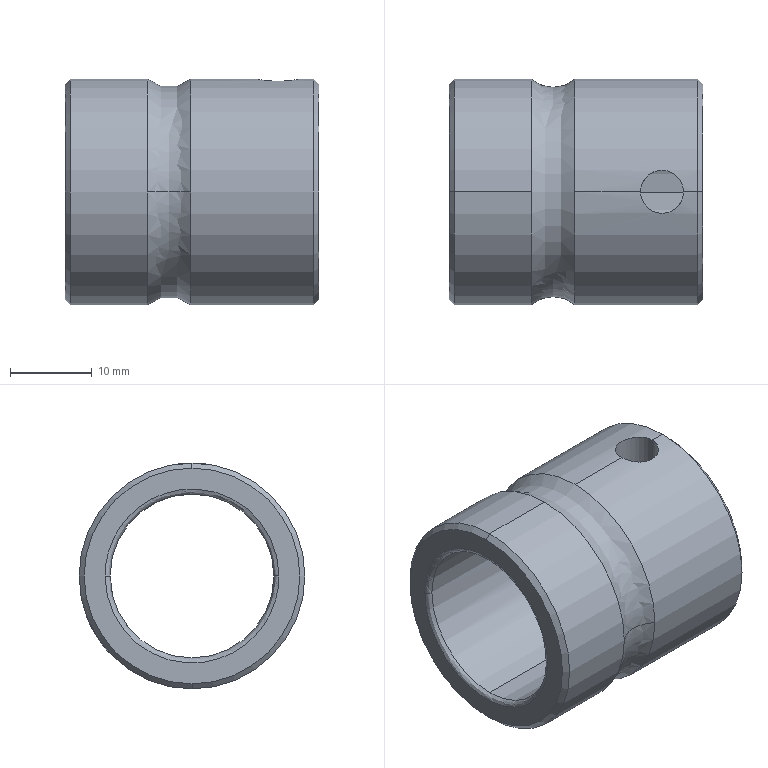Part | STEP file | Microwave Drying Flat Conveyor-inafag_ucfl204_62o9y6gnj3059x015y4y3bh4_03 | 1 solid | 22 faces | box 31 x 27.56 x 27.56 mm | volume 8243 mm3 | cylinder 10 | spline 6 | cone 4 | plane 2 | commonest cylinder face diameters 5.25 x4 27.56 x4 20 x2
STEP:
#1=CARTESIAN_POINT('',(2.3,10.62,0.));
#2=VERTEX_POINT('',#1);
#3=CARTESIAN_POINT('',(2.3,-10.62,0.));
#4=VERTEX_POINT('',#3);
#5=CARTESIAN_POINT('',(2.3,10.62,0.));
#6=CARTESIAN_POINT('',(2.3,10.62,-21.24));
#7=CARTESIAN_POINT('',(2.3,-10.62,-21.24));
#8=CARTESIAN_POINT('',(2.3,-10.62,0.));
#9=(BOUNDED_CURVE()B_SPLINE_CURVE(3,(#5,#6,#7,#8),.UNSPECIFIED.,.F.,.F.)B_SPLINE_CURVE_WITH_KNOTS((4,4),(0.25,0.75),.UNSPECIFIED.)CURVE()GEOMETRIC_REPRESENTATION_ITEM()RATIONAL_B_SPLINE_CURVE((1.,0.3333,0.3333,1.))REPRESENTATION_ITEM(''));
#10=EDGE_CURVE('',#2,#4,#9,.T.);
#11=ORIENTED_EDGE('',*,*,#10,.T.);
#12=CARTESIAN_POINT('',(2.92,-10.,0.));
#13=VERTEX_POINT('',#12);
#14=CARTESIAN_POINT('',(2.92,-10.62,0.));
#15=DIRECTION('',(0.,0.,-1.));
#16=DIRECTION('',(0.,-1.,0.));
#17=AXIS2_PLACEMENT_3D('',#14,#15,#16);
#18=CIRCLE('',#17,0.62);
#19=EDGE_CURVE('',#4,#13,#18,.T.);
#20=ORIENTED_EDGE('',*,*,#19,.T.);
#21=CARTESIAN_POINT('',(2.92,0.,-10.));
#22=VERTEX_POINT('',#21);
#23=CARTESIAN_POINT('',(2.92,0.,0.));
#24=DIRECTION('',(-1.,0.,0.));
#25=DIRECTION('',(0.,0.,1.));
#26=AXIS2_PLACEMENT_3D('',#23,#24,#25);
#27=CIRCLE('',#26,10.);
#28=EDGE_CURVE('',#22,#13,#27,.T.);
#29=ORIENTED_EDGE('',*,*,#28,.F.);
#30=CARTESIAN_POINT('',(2.92,10.,0.));
#31=VERTEX_POINT('',#30);
#32=CARTESIAN_POINT('',(2.92,0.,0.));
#33=DIRECTION('',(-1.,0.,0.));
#34=DIRECTION('',(0.,0.,1.));
#35=AXIS2_PLACEMENT_3D('',#32,#33,#34);
#36=CIRCLE('',#35,10.);
#37=EDGE_CURVE('',#31,#22,#36,.T.);
#38=ORIENTED_EDGE('',*,*,#37,.F.);
#39=CARTESIAN_POINT('',(2.92,10.62,0.));
#40=DIRECTION('',(0.,0.,1.));
#41=DIRECTION('',(0.,1.,0.));
#42=AXIS2_PLACEMENT_3D('',#39,#40,#41);
#43=CIRCLE('',#42,0.62);
#44=EDGE_CURVE('',#2,#31,#43,.T.);
#45=ORIENTED_EDGE('',*,*,#44,.F.);
#46=EDGE_LOOP('',(#11,#20,#29,#38,#45));
#47=FACE_OUTER_BOUND('',#46,.T.);
#48=CARTESIAN_POINT('',(2.3,-10.62,0.));
#49=CARTESIAN_POINT('',(2.3,-10.62,-21.24));
#50=CARTESIAN_POINT('',(2.3,10.62,-21.24));
#51=CARTESIAN_POINT('',(2.3,10.62,0.));
#52=CARTESIAN_POINT('',(2.3,-10.257,0.));
#53=CARTESIAN_POINT('',(2.3,-10.257,-20.514));
#54=CARTESIAN_POINT('',(2.3,10.257,-20.514));
#55=CARTESIAN_POINT('',(2.3,10.257,0.));
#56=CARTESIAN_POINT('',(2.557,-10.,0.));
#57=CARTESIAN_POINT('',(2.557,-10.,-20.));
#58=CARTESIAN_POINT('',(2.557,10.,-20.));
#59=CARTESIAN_POINT('',(2.557,10.,0.));
#60=CARTESIAN_POINT('',(2.92,-10.,0.));
#61=CARTESIAN_POINT('',(2.92,-10.,-20.));
#62=CARTESIAN_POINT('',(2.92,10.,-20.));
#63=CARTESIAN_POINT('',(2.92,10.,0.));
#64=(BOUNDED_SURFACE()B_SPLINE_SURFACE(3,3,((#48,#49,#50,#51),(#52,#53,#54,#55),(#56,#57,#58,#59),(#60,#61,#62,#63)),.UNSPECIFIED.,.F.,.F.,.T.)B_SPLINE_SURFACE_WITH_KNOTS((4,4),(4,4),(0.,1.),(0.,1.),.UNSPECIFIED.)GEOMETRIC_REPRESENTATION_ITEM()RATIONAL_B_SPLINE_SURFACE(((1.,0.3333,0.3333,1.),(0.8047,0.2682,0.2682,0.8047),(0.8047,0.2682,0.2682,0.8047),(1.,0.3333,0.3333,1.)))REPRESENTATION_ITEM('')SURFACE());
#65=ADVANCED_FACE('',(#47),#64,.T.);
#66=CARTESIAN_POINT('',(32.68,-10.,0.));
#67=VERTEX_POINT('',#66);
#68=CARTESIAN_POINT('',(32.68,0.,-10.));
#69=VERTEX_POINT('',#68);
#70=CARTESIAN_POINT('',(32.68,0.,0.));
#71=DIRECTION('',(1.,0.,0.));
#72=DIRECTION('',(0.,0.,1.));
#73=AXIS2_PLACEMENT_3D('',#70,#71,#72);
#74=CIRCLE('',#73,10.);
#75=EDGE_CURVE('',#67,#69,#74,.T.);
#76=ORIENTED_EDGE('',*,*,#75,.F.);
#77=CARTESIAN_POINT('',(33.3,-10.62,0.));
#78=VERTEX_POINT('',#77);
#79=CARTESIAN_POINT('',(32.68,-10.62,0.));
#80=DIRECTION('',(0.,0.,-1.));
#81=DIRECTION('',(0.,-1.,0.));
#82=AXIS2_PLACEMENT_3D('',#79,#80,#81);
#83=CIRCLE('',#82,0.62);
#84=EDGE_CURVE('',#67,#78,#83,.T.);
#85=ORIENTED_EDGE('',*,*,#84,.T.);
#86=CARTESIAN_POINT('',(33.3,10.62,0.));
#87=VERTEX_POINT('',#86);
#88=CARTESIAN_POINT('',(33.3,-10.62,0.));
#89=CARTESIAN_POINT('',(33.3,-10.62,-21.24));
#90=CARTESIAN_POINT('',(33.3,10.62,-21.24));
#91=CARTESIAN_POINT('',(33.3,10.62,0.));
#92=(BOUNDED_CURVE()B_SPLINE_CURVE(3,(#88,#89,#90,#91),.UNSPECIFIED.,.F.,.F.)B_SPLINE_CURVE_WITH_KNOTS((4,4),(0.25,0.75),.UNSPECIFIED.)CURVE()GEOMETRIC_REPRESENTATION_ITEM()RATIONAL_B_SPLINE_CURVE((1.,0.3333,0.3333,1.))REPRESENTATION_ITEM(''));
#93=EDGE_CURVE('',#78,#87,#92,.T.);
#94=ORIENTED_EDGE('',*,*,#93,.T.);
#95=CARTESIAN_POINT('',(32.68,10.,0.));
#96=VERTEX_POINT('',#95);
#97=CARTESIAN_POINT('',(32.68,10.62,0.));
#98=DIRECTION('',(0.,0.,1.));
#99=DIRECTION('',(0.,1.,0.));
#100=AXIS2_PLACEMENT_3D('',#97,#98,#99);
#101=CIRCLE('',#100,0.62);
#102=EDGE_CURVE('',#96,#87,#101,.T.);
#103=ORIENTED_EDGE('',*,*,#102,.F.);
#104=CARTESIAN_POINT('',(32.68,0.,0.));
#105=DIRECTION('',(1.,0.,0.));
#106=DIRECTION('',(0.,0.,1.));
#107=AXIS2_PLACEMENT_3D('',#104,#105,#106);
#108=CIRCLE('',#107,10.);
#109=EDGE_CURVE('',#69,#96,#108,.T.);
#110=ORIENTED_EDGE('',*,*,#109,.F.);
#111=EDGE_LOOP('',(#76,#85,#94,#103,#110));
#112=FACE_OUTER_BOUND('',#111,.T.);
#113=CARTESIAN_POINT('',(32.68,-10.,0.));
#114=CARTESIAN_POINT('',(32.68,-10.,-20.));
#115=CARTESIAN_POINT('',(32.68,10.,-20.));
#116=CARTESIAN_POINT('',(32.68,10.,0.));
#117=CARTESIAN_POINT('',(33.043,-10.,0.));
#118=CARTESIAN_POINT('',(33.043,-10.,-20.));
#119=CARTESIAN_POINT('',(33.043,10.,-20.));
#120=CARTESIAN_POINT('',(33.043,10.,0.));
#121=CARTESIAN_POINT('',(33.3,-10.257,0.));
#122=CARTESIAN_POINT('',(33.3,-10.257,-20.514));
#123=CARTESIAN_POINT('',(33.3,10.257,-20.514));
#124=CARTESIAN_POINT('',(33.3,10.257,0.));
#125=CARTESIAN_POINT('',(33.3,-10.62,0.));
#126=CARTESIAN_POINT('',(33.3,-10.62,-21.24));
#127=CARTESIAN_POINT('',(33.3,10.62,-21.24));
#128=CARTESIAN_POINT('',(33.3,10.62,0.));
#129=(BOUNDED_SURFACE()B_SPLINE_SURFACE(3,3,((#113,#114,#115,#116),(#117,#118,#119,#120),(#121,#122,#123,#124),(#125,#126,#127,#128)),.UNSPECIFIED.,.F.,.F.,.F.)B_SPLINE_SURFACE_WITH_KNOTS((4,4),(4,4),(0.,1.),(0.,1.),.UNSPECIFIED.)GEOMETRIC_REPRESENTATION_ITEM()RATIONAL_B_SPLINE_SURFACE(((1.,0.3333,0.3333,1.),(0.8047,0.2682,0.2682,0.8047),(0.8047,0.2682,0.2682,0.8047),(1.,0.3333,0.3333,1.)))REPRESENTATION_ITEM('')SURFACE());
#130=ADVANCED_FACE('',(#112),#129,.T.);
#131=CARTESIAN_POINT('',(17.634,-13.78,0.));
#132=VERTEX_POINT('',#131);
#133=CARTESIAN_POINT('',(17.634,0.,-13.78));
#134=VERTEX_POINT('',#133);
#135=CARTESIAN_POINT('',(17.634,0.,0.));
#136=DIRECTION('',(1.,0.,0.));
#137=DIRECTION('',(0.,0.,-1.));
#138=AXIS2_PLACEMENT_3D('',#135,#136,#137);
#139=CIRCLE('',#138,13.78);
#140=EDGE_CURVE('',#132,#134,#139,.T.);
#141=ORIENTED_EDGE('',*,*,#140,.F.);
#142=CARTESIAN_POINT('',(12.366,-13.78,0.));
#143=VERTEX_POINT('',#142);
#144=CARTESIAN_POINT('',(15.,-16.75,0.));
#145=DIRECTION('',(0.,0.,1.));
#146=DIRECTION('',(0.,-1.,0.));
#147=AXIS2_PLACEMENT_3D('',#144,#145,#146);
#148=CIRCLE('',#147,3.97);
#149=EDGE_CURVE('',#132,#143,#148,.T.);
#150=ORIENTED_EDGE('',*,*,#149,.T.);
#151=CARTESIAN_POINT('',(12.366,0.,-13.78));
#152=VERTEX_POINT('',#151);
#153=CARTESIAN_POINT('',(12.366,0.,0.));
#154=DIRECTION('',(1.,0.,0.));
#155=DIRECTION('',(0.,1.,0.));
#156=AXIS2_PLACEMENT_3D('',#153,#154,#155);
#157=CIRCLE('',#156,13.78);
#158=EDGE_CURVE('',#143,#152,#157,.T.);
#159=ORIENTED_EDGE('',*,*,#158,.T.);
#160=CARTESIAN_POINT('',(12.366,13.78,0.));
#161=VERTEX_POINT('',#160);
#162=CARTESIAN_POINT('',(12.366,0.,0.));
#163=DIRECTION('',(1.,0.,0.));
#164=DIRECTION('',(0.,1.,0.));
#165=AXIS2_PLACEMENT_3D('',#162,#163,#164);
#166=CIRCLE('',#165,13.78);
#167=EDGE_CURVE('',#152,#161,#166,.T.);
#168=ORIENTED_EDGE('',*,*,#167,.T.);
#169=CARTESIAN_POINT('',(17.634,13.78,0.));
#170=VERTEX_POINT('',#169);
#171=CARTESIAN_POINT('',(15.,16.75,0.));
#172=DIRECTION('',(0.,0.,-1.));
#173=DIRECTION('',(0.,1.,0.));
#174=AXIS2_PLACEMENT_3D('',#171,#172,#173);
#175=CIRCLE('',#174,3.97);
#176=EDGE_CURVE('',#170,#161,#175,.T.);
#177=ORIENTED_EDGE('',*,*,#176,.F.);
#178=CARTESIAN_POINT('',(17.634,0.,0.));
#179=DIRECTION('',(1.,0.,0.));
#180=DIRECTION('',(0.,0.,-1.));
#181=AXIS2_PLACEMENT_3D('',#178,#179,#180);
#182=CIRCLE('',#181,13.78);
#183=EDGE_CURVE('',#134,#170,#182,.T.);
#184=ORIENTED_EDGE('',*,*,#183,.F.);
#185=EDGE_LOOP('',(#141,#150,#159,#168,#177,#184));
#186=FACE_OUTER_BOUND('',#185,.T.);
#187=CARTESIAN_POINT('',(17.634,-13.78,0.));
#188=CARTESIAN_POINT('',(17.634,-13.78,-27.56));
#189=CARTESIAN_POINT('',(17.634,13.78,-27.56));
#190=CARTESIAN_POINT('',(17.634,13.78,0.));
#191=CARTESIAN_POINT('',(16.055,-12.379,0.));
#192=CARTESIAN_POINT('',(16.055,-12.379,-24.759));
#193=CARTESIAN_POINT('',(16.055,12.379,-24.759));
#194=CARTESIAN_POINT('',(16.055,12.379,0.));
#195=CARTESIAN_POINT('',(13.945,-12.379,0.));
#196=CARTESIAN_POINT('',(13.945,-12.379,-24.759));
#197=CARTESIAN_POINT('',(13.945,12.379,-24.759));
#198=CARTESIAN_POINT('',(13.945,12.379,0.));
#199=CARTESIAN_POINT('',(12.366,-13.78,0.));
#200=CARTESIAN_POINT('',(12.366,-13.78,-27.56));
#201=CARTESIAN_POINT('',(12.366,13.78,-27.56));
#202=CARTESIAN_POINT('',(12.366,13.78,0.));
#203=(BOUNDED_SURFACE()B_SPLINE_SURFACE(3,3,((#187,#188,#189,#190),(#191,#192,#193,#194),(#195,#196,#197,#198),(#199,#200,#201,#202)),.UNSPECIFIED.,.F.,.F.,.F.)B_SPLINE_SURFACE_WITH_KNOTS((4,4),(4,4),(0.,1.),(0.,1.),.UNSPECIFIED.)GEOMETRIC_REPRESENTATION_ITEM()RATIONAL_B_SPLINE_SURFACE(((1.,0.3333,0.3333,1.),(0.8321,0.2774,0.2774,0.8321),(0.8321,0.2774,0.2774,0.8321),(1.,0.3333,0.3333,1.)))REPRESENTATION_ITEM('')SURFACE());
#204=ADVANCED_FACE('',(#186),#203,.T.);
#205=ORIENTED_EDGE('',*,*,#28,.T.);
#206=CARTESIAN_POINT('',(2.92,0.,10.));
#207=VERTEX_POINT('',#206);
#208=CARTESIAN_POINT('',(2.92,0.,0.));
#209=DIRECTION('',(-1.,0.,0.));
#210=DIRECTION('',(0.,0.,1.));
#211=AXIS2_PLACEMENT_3D('',#208,#209,#210);
#212=CIRCLE('',#211,10.);
#213=EDGE_CURVE('',#13,#207,#212,.T.);
#214=ORIENTED_EDGE('',*,*,#213,.T.);
#215=CARTESIAN_POINT('',(25.675,0.,10.));
#216=VERTEX_POINT('',#215);
#217=CARTESIAN_POINT('',(2.92,0.,10.));
#218=DIRECTION('',(1.,0.,0.));
#219=VECTOR('',#218,1000.);
#220=LINE('',#217,#219);
#221=EDGE_CURVE('',#207,#216,#220,.T.);
#222=ORIENTED_EDGE('',*,*,#221,.T.);
#223=CARTESIAN_POINT('',(30.925,0.,10.));
#224=VERTEX_POINT('',#223);
#225=CARTESIAN_POINT('',(25.675,0.,10.));
#226=CARTESIAN_POINT('',(25.675,-0.1741,10.));
#227=CARTESIAN_POINT('',(25.692,-0.3452,9.995));
#228=CARTESIAN_POINT('',(25.759,-0.6816,9.978));
#229=CARTESIAN_POINT('',(25.81,-0.8487,9.965));
#230=CARTESIAN_POINT('',(25.942,-1.166,9.933));
#231=CARTESIAN_POINT('',(26.023,-1.317,9.914));
#232=CARTESIAN_POINT('',(26.213,-1.601,9.872));
#233=CARTESIAN_POINT('',(26.323,-1.735,9.849));
#234=CARTESIAN_POINT('',(26.684,-2.097,9.781));
#235=CARTESIAN_POINT('',(26.976,-2.292,9.735));
#236=CARTESIAN_POINT('',(27.448,-2.489,9.686));
#237=CARTESIAN_POINT('',(27.614,-2.54,9.672));
#238=CARTESIAN_POINT('',(27.954,-2.608,9.654));
#239=CARTESIAN_POINT('',(28.126,-2.625,9.649));
#240=CARTESIAN_POINT('',(28.474,-2.625,9.649));
#241=CARTESIAN_POINT('',(28.645,-2.608,9.654));
#242=CARTESIAN_POINT('',(28.982,-2.541,9.672));
#243=CARTESIAN_POINT('',(29.149,-2.49,9.685));
#244=CARTESIAN_POINT('',(29.466,-2.358,9.718));
#245=CARTESIAN_POINT('',(29.616,-2.278,9.738));
#246=CARTESIAN_POINT('',(29.901,-2.087,9.78));
#247=CARTESIAN_POINT('',(30.035,-1.977,9.803));
#248=CARTESIAN_POINT('',(30.397,-1.616,9.872));
#249=CARTESIAN_POINT('',(30.592,-1.325,9.917));
#250=CARTESIAN_POINT('',(30.789,-0.8516,9.965));
#251=CARTESIAN_POINT('',(30.84,-0.6858,9.978));
#252=CARTESIAN_POINT('',(30.908,-0.3461,9.995));
#253=CARTESIAN_POINT('',(30.925,-0.1741,10.));
#254=CARTESIAN_POINT('',(30.925,0.,10.));
#255=B_SPLINE_CURVE_WITH_KNOTS('',3,(#225,#226,#227,#228,#229,#230,#231,#232,#233,#234,#235,#236,#237,#238,#239,#240,#241,#242,#243,#244,#245,#246,#247,#248,#249,#250,#251,#252,#253,#254),.UNSPECIFIED.,.F.,.F.,(4,2,2,2,2,2,2,2,2,2,2,2,2,2,4),(0.,0.0005149,0.00103,0.001545,0.002059,0.003089,0.003604,0.004119,0.004634,0.005149,0.005663,0.006178,0.007208,0.007723,0.008238),.UNSPECIFIED.);
#256=EDGE_CURVE('',#216,#224,#255,.T.);
#257=ORIENTED_EDGE('',*,*,#256,.T.);
#258=CARTESIAN_POINT('',(32.68,0.,10.));
#259=VERTEX_POINT('',#258);
#260=CARTESIAN_POINT('',(2.92,0.,10.));
#261=DIRECTION('',(1.,0.,0.));
#262=VECTOR('',#261,1000.);
#263=LINE('',#260,#262);
#264=EDGE_CURVE('',#224,#259,#263,.T.);
#265=ORIENTED_EDGE('',*,*,#264,.T.);
#266=CARTESIAN_POINT('',(32.68,0.,0.));
#267=DIRECTION('',(1.,0.,0.));
#268=DIRECTION('',(0.,0.,1.));
#269=AXIS2_PLACEMENT_3D('',#266,#267,#268);
#270=CIRCLE('',#269,10.);
#271=EDGE_CURVE('',#259,#67,#270,.T.);
#272=ORIENTED_EDGE('',*,*,#271,.T.);
#273=ORIENTED_EDGE('',*,*,#75,.T.);
#274=CARTESIAN_POINT('',(2.92,0.,-10.));
#275=DIRECTION('',(1.,0.,0.));
#276=VECTOR('',#275,1000.);
#277=LINE('',#274,#276);
#278=EDGE_CURVE('',#22,#69,#277,.T.);
#279=ORIENTED_EDGE('',*,*,#278,.F.);
#280=EDGE_LOOP('',(#205,#214,#222,#257,#265,#272,#273,#279));
#281=FACE_OUTER_BOUND('',#280,.T.);
#282=CARTESIAN_POINT('',(2.92,0.,0.));
#283=DIRECTION('',(1.,0.,0.));
#284=DIRECTION('',(0.,0.,-1.));
#285=AXIS2_PLACEMENT_3D('',#282,#283,#284);
#286=CYLINDRICAL_SURFACE('',#285,10.);
#287=ADVANCED_FACE('',(#281),#286,.F.);
#288=ORIENTED_EDGE('',*,*,#256,.F.);
#289=CARTESIAN_POINT('',(25.675,0.,13.78));
#290=VERTEX_POINT('',#289);
#291=CARTESIAN_POINT('',(25.675,0.,13.78));
#292=DIRECTION('',(0.,0.,1.));
#293=VECTOR('',#292,1000.);
#294=LINE('',#291,#293);
#295=EDGE_CURVE('',#216,#290,#294,.T.);
#296=ORIENTED_EDGE('',*,*,#295,.T.);
#297=CARTESIAN_POINT('',(30.925,0.,13.78));
#298=VERTEX_POINT('',#297);
#299=CARTESIAN_POINT('',(30.925,0.,13.78));
#300=CARTESIAN_POINT('',(30.925,-0.1737,13.78));
#301=CARTESIAN_POINT('',(30.908,-0.3445,13.777));
#302=CARTESIAN_POINT('',(30.841,-0.6804,13.764));
#303=CARTESIAN_POINT('',(30.79,-0.8472,13.755));
#304=CARTESIAN_POINT('',(30.659,-1.165,13.732));
#305=CARTESIAN_POINT('',(30.578,-1.315,13.718));
#306=CARTESIAN_POINT('',(30.388,-1.6,13.688));
#307=CARTESIAN_POINT('',(30.277,-1.735,13.671));
#308=CARTESIAN_POINT('',(30.036,-1.976,13.638));
#309=CARTESIAN_POINT('',(29.904,-2.085,13.622));
#310=CARTESIAN_POINT('',(29.618,-2.277,13.591));
#311=CARTESIAN_POINT('',(29.466,-2.358,13.577));
#312=CARTESIAN_POINT('',(28.993,-2.555,13.542));
#313=CARTESIAN_POINT('',(28.648,-2.625,13.528));
#314=CARTESIAN_POINT('',(28.126,-2.625,13.528));
#315=CARTESIAN_POINT('',(27.956,-2.608,13.531));
#316=CARTESIAN_POINT('',(27.62,-2.541,13.544));
#317=CARTESIAN_POINT('',(27.453,-2.49,13.553));
#318=CARTESIAN_POINT('',(27.135,-2.359,13.577));
#319=CARTESIAN_POINT('',(26.985,-2.278,13.591));
#320=CARTESIAN_POINT('',(26.7,-2.088,13.621));
#321=CARTESIAN_POINT('',(26.565,-1.977,13.638));
#322=CARTESIAN_POINT('',(26.324,-1.736,13.671));
#323=CARTESIAN_POINT('',(26.215,-1.604,13.687));
#324=CARTESIAN_POINT('',(26.023,-1.318,13.718));
#325=CARTESIAN_POINT('',(25.942,-1.166,13.732));
#326=CARTESIAN_POINT('',(25.745,-0.6926,13.766));
#327=CARTESIAN_POINT('',(25.675,-0.3475,13.78));
#328=CARTESIAN_POINT('',(25.675,0.,13.78));
#329=B_SPLINE_CURVE_WITH_KNOTS('',3,(#299,#300,#301,#302,#303,#304,#305,#306,#307,#308,#309,#310,#311,#312,#313,#314,#315,#316,#317,#318,#319,#320,#321,#322,#323,#324,#325,#326,#327,#328),.UNSPECIFIED.,.F.,.F.,(4,2,2,2,2,2,2,2,2,2,2,2,2,2,4),(0.01233,0.01285,0.01336,0.01388,0.01439,0.0149,0.01542,0.01644,0.01696,0.01747,0.01799,0.0185,0.01901,0.01953,0.02055),.UNSPECIFIED.);
#330=EDGE_CURVE('',#298,#290,#329,.T.);
#331=ORIENTED_EDGE('',*,*,#330,.F.);
#332=CARTESIAN_POINT('',(30.925,0.,13.78));
#333=DIRECTION('',(0.,0.,1.));
#334=VECTOR('',#333,1000.);
#335=LINE('',#332,#334);
#336=EDGE_CURVE('',#224,#298,#335,.T.);
#337=ORIENTED_EDGE('',*,*,#336,.F.);
#338=EDGE_LOOP('',(#288,#296,#331,#337));
#339=FACE_OUTER_BOUND('',#338,.T.);
#340=CARTESIAN_POINT('',(28.3,0.,13.78));
#341=DIRECTION('',(0.,0.,1.));
#342=DIRECTION('',(1.,0.,0.));
#343=AXIS2_PLACEMENT_3D('',#340,#341,#342);
#344=CYLINDRICAL_SURFACE('',#343,2.625);
#345=ADVANCED_FACE('',(#339),#344,.F.);
#346=CARTESIAN_POINT('',(28.3,7.044,-7.098));
#347=VERTEX_POINT('',#346);
#348=CARTESIAN_POINT('',(28.3,9.669,-2.551));
#349=VERTEX_POINT('',#348);
#350=CARTESIAN_POINT('',(28.3,7.044,-7.098));
#351=CARTESIAN_POINT('',(28.128,7.044,-7.098));
#352=CARTESIAN_POINT('',(27.953,7.057,-7.085));
#353=CARTESIAN_POINT('',(27.616,7.106,-7.036));
#354=CARTESIAN_POINT('',(27.453,7.142,-6.999));
#355=CARTESIAN_POINT('',(26.975,7.285,-6.852));
#356=CARTESIAN_POINT('',(26.687,7.421,-6.708));
#357=CARTESIAN_POINT('',(26.322,7.662,-6.427));
#358=CARTESIAN_POINT('',(26.214,7.748,-6.324));
#359=CARTESIAN_POINT('',(26.024,7.926,-6.1));
#360=CARTESIAN_POINT('',(25.942,8.019,-5.976));
#361=CARTESIAN_POINT('',(25.81,8.205,-5.718));
#362=CARTESIAN_POINT('',(25.76,8.298,-5.583));
#363=CARTESIAN_POINT('',(25.692,8.482,-5.299));
#364=CARTESIAN_POINT('',(25.675,8.573,-5.15));
#365=CARTESIAN_POINT('',(25.675,8.748,-4.849));
#366=CARTESIAN_POINT('',(25.692,8.829,-4.698));
#367=CARTESIAN_POINT('',(25.759,8.982,-4.399));
#368=CARTESIAN_POINT('',(25.81,9.055,-4.247));
#369=CARTESIAN_POINT('',(25.942,9.185,-3.956));
#370=CARTESIAN_POINT('',(26.023,9.244,-3.817));
#371=CARTESIAN_POINT('',(26.213,9.35,-3.549));
#372=CARTESIAN_POINT('',(26.323,9.397,-3.422));
#373=CARTESIAN_POINT('',(26.684,9.519,-3.075));
#374=CARTESIAN_POINT('',(26.976,9.577,-2.882));
#375=CARTESIAN_POINT('',(27.448,9.632,-2.687));
#376=CARTESIAN_POINT('',(27.614,9.646,-2.637));
#377=CARTESIAN_POINT('',(27.954,9.665,-2.569));
#378=CARTESIAN_POINT('',(28.126,9.669,-2.551));
#379=CARTESIAN_POINT('',(28.3,9.669,-2.551));
#380=B_SPLINE_CURVE_WITH_KNOTS('',3,(#350,#351,#352,#353,#354,#355,#356,#357,#358,#359,#360,#361,#362,#363,#364,#365,#366,#367,#368,#369,#370,#371,#372,#373,#374,#375,#376,#377,#378,#379),.UNSPECIFIED.,.F.,.F.,(4,2,2,2,2,2,2,2,2,2,2,2,2,2,4),(-0.004118,-0.003603,-0.003088,-0.002059,-0.001544,-0.001029,-0.0005144,0.000000397,0.0005152,0.00103,0.001545,0.00206,0.003089,0.003604,0.004119),.UNSPECIFIED.);
#381=EDGE_CURVE('',#347,#349,#380,.T.);
#382=ORIENTED_EDGE('',*,*,#381,.F.);
#383=CARTESIAN_POINT('',(28.3,10.403,-9.037));
#384=VERTEX_POINT('',#383);
#385=CARTESIAN_POINT('',(28.3,10.621,-9.163));
#386=DIRECTION('',(0.,0.866,-0.5));
#387=VECTOR('',#386,1000.);
#388=LINE('',#385,#387);
#389=EDGE_CURVE('',#347,#384,#388,.T.);
#390=ORIENTED_EDGE('',*,*,#389,.T.);
#391=CARTESIAN_POINT('',(28.3,13.028,-4.491));
#392=VERTEX_POINT('',#391);
#393=CARTESIAN_POINT('',(28.3,13.028,-4.491));
#394=CARTESIAN_POINT('',(28.126,13.028,-4.491));
#395=CARTESIAN_POINT('',(27.955,13.022,-4.507));
#396=CARTESIAN_POINT('',(27.619,13.,-4.571));
#397=CARTESIAN_POINT('',(27.452,12.983,-4.62));
#398=CARTESIAN_POINT('',(27.135,12.937,-4.746));
#399=CARTESIAN_POINT('',(26.984,12.909,-4.823));
#400=CARTESIAN_POINT('',(26.699,12.84,-5.003));
#401=CARTESIAN_POINT('',(26.564,12.799,-5.107));
#402=CARTESIAN_POINT('',(26.323,12.707,-5.333));
#403=CARTESIAN_POINT('',(26.214,12.655,-5.455));
#404=CARTESIAN_POINT('',(26.023,12.538,-5.719));
#405=CARTESIAN_POINT('',(25.941,12.474,-5.857));
#406=CARTESIAN_POINT('',(25.745,12.267,-6.285));
#407=CARTESIAN_POINT('',(25.675,12.107,-6.591));
#408=CARTESIAN_POINT('',(25.675,11.846,-7.042));
#409=CARTESIAN_POINT('',(25.692,11.758,-7.189));
#410=CARTESIAN_POINT('',(25.76,11.579,-7.473));
#411=CARTESIAN_POINT('',(25.81,11.487,-7.613));
#412=CARTESIAN_POINT('',(25.942,11.308,-7.876));
#413=CARTESIAN_POINT('',(26.023,11.221,-8.));
#414=CARTESIAN_POINT('',(26.214,11.052,-8.231));
#415=CARTESIAN_POINT('',(26.324,10.971,-8.34));
#416=CARTESIAN_POINT('',(26.566,10.822,-8.532));
#417=CARTESIAN_POINT('',(26.698,10.753,-8.618));
#418=CARTESIAN_POINT('',(26.985,10.631,-8.769));
#419=CARTESIAN_POINT('',(27.137,10.578,-8.832));
#420=CARTESIAN_POINT('',(27.453,10.492,-8.933));
#421=CARTESIAN_POINT('',(27.619,10.459,-8.972));
#422=CARTESIAN_POINT('',(27.958,10.414,-9.024));
#423=CARTESIAN_POINT('',(28.128,10.403,-9.037));
#424=CARTESIAN_POINT('',(28.3,10.403,-9.037));
#425=B_SPLINE_CURVE_WITH_KNOTS('',3,(#393,#394,#395,#396,#397,#398,#399,#400,#401,#402,#403,#404,#405,#406,#407,#408,#409,#410,#411,#412,#413,#414,#415,#416,#417,#418,#419,#420,#421,#422,#423,#424),.UNSPECIFIED.,.F.,.F.,(4,2,2,2,2,2,2,2,2,2,2,2,2,2,2,4),(0.,0.000514,0.001028,0.001542,0.002056,0.00257,0.003084,0.004112,0.004626,0.00514,0.005654,0.006168,0.006682,0.007196,0.00771,0.008224),.UNSPECIFIED.);
#426=EDGE_CURVE('',#392,#384,#425,.T.);
#427=ORIENTED_EDGE('',*,*,#426,.F.);
#428=CARTESIAN_POINT('',(28.3,13.246,-4.617));
#429=DIRECTION('',(0.,0.866,-0.5));
#430=VECTOR('',#429,1000.);
#431=LINE('',#428,#430);
#432=EDGE_CURVE('',#349,#392,#431,.T.);
#433=ORIENTED_EDGE('',*,*,#432,.F.);
#434=EDGE_LOOP('',(#382,#390,#427,#433));
#435=FACE_OUTER_BOUND('',#434,.T.);
#436=CARTESIAN_POINT('',(28.3,11.934,-6.89));
#437=DIRECTION('',(0.,0.866,-0.5));
#438=DIRECTION('',(0.,0.5,0.866));
#439=AXIS2_PLACEMENT_3D('',#436,#437,#438);
#440=CYLINDRICAL_SURFACE('',#439,2.625);
#441=ADVANCED_FACE('',(#435),#440,.F.);
#442=ORIENTED_EDGE('',*,*,#426,.T.);
#443=CARTESIAN_POINT('',(28.3,10.403,-9.037));
#444=CARTESIAN_POINT('',(28.472,10.403,-9.037));
#445=CARTESIAN_POINT('',(28.646,10.414,-9.024));
#446=CARTESIAN_POINT('',(28.983,10.459,-8.972));
#447=CARTESIAN_POINT('',(29.146,10.492,-8.934));
#448=CARTESIAN_POINT('',(29.464,10.578,-8.831));
#449=CARTESIAN_POINT('',(29.617,10.632,-8.767));
#450=CARTESIAN_POINT('',(29.901,10.753,-8.618));
#451=CARTESIAN_POINT('',(30.034,10.822,-8.532));
#452=CARTESIAN_POINT('',(30.278,10.972,-8.338));
#453=CARTESIAN_POINT('',(30.386,11.052,-8.231));
#454=CARTESIAN_POINT('',(30.576,11.22,-8.001));
#455=CARTESIAN_POINT('',(30.659,11.309,-7.875));
#456=CARTESIAN_POINT('',(30.79,11.488,-7.612));
#457=CARTESIAN_POINT('',(30.84,11.578,-7.475));
#458=CARTESIAN_POINT('',(30.908,11.757,-7.189));
#459=CARTESIAN_POINT('',(30.925,11.847,-7.04));
#460=CARTESIAN_POINT('',(30.925,12.021,-6.739));
#461=CARTESIAN_POINT('',(30.908,12.103,-6.59));
#462=CARTESIAN_POINT('',(30.841,12.26,-6.293));
#463=CARTESIAN_POINT('',(30.79,12.336,-6.144));
#464=CARTESIAN_POINT('',(30.659,12.474,-5.857));
#465=CARTESIAN_POINT('',(30.578,12.538,-5.72));
#466=CARTESIAN_POINT('',(30.388,12.654,-5.458));
#467=CARTESIAN_POINT('',(30.277,12.707,-5.333));
#468=CARTESIAN_POINT('',(30.036,12.799,-5.107));
#469=CARTESIAN_POINT('',(29.904,12.839,-5.005));
#470=CARTESIAN_POINT('',(29.618,12.909,-4.824));
#471=CARTESIAN_POINT('',(29.466,12.937,-4.746));
#472=CARTESIAN_POINT('',(28.993,13.005,-4.558));
#473=CARTESIAN_POINT('',(28.647,13.028,-4.491));
#474=CARTESIAN_POINT('',(28.3,13.028,-4.491));
#475=B_SPLINE_CURVE_WITH_KNOTS('',3,(#443,#444,#445,#446,#447,#448,#449,#450,#451,#452,#453,#454,#455,#456,#457,#458,#459,#460,#461,#462,#463,#464,#465,#466,#467,#468,#469,#470,#471,#472,#473,#474),.UNSPECIFIED.,.F.,.F.,(4,2,2,2,2,2,2,2,2,2,2,2,2,2,2,4),(0.008224,0.008738,0.009252,0.009765,0.01028,0.01079,0.01131,0.01182,0.01233,0.01285,0.01336,0.01388,0.01439,0.0149,0.01542,0.01644),.UNSPECIFIED.);
#476=EDGE_CURVE('',#384,#392,#475,.T.);
#477=ORIENTED_EDGE('',*,*,#476,.T.);
#478=EDGE_LOOP('',(#442,#477));
#479=FACE_BOUND('',#478,.T.);
#480=ORIENTED_EDGE('',*,*,#183,.T.);
#481=CARTESIAN_POINT('',(17.634,0.,13.78));
#482=VERTEX_POINT('',#481);
#483=CARTESIAN_POINT('',(17.634,0.,0.));
#484=DIRECTION('',(1.,0.,0.));
#485=DIRECTION('',(0.,0.,-1.));
#486=AXIS2_PLACEMENT_3D('',#483,#484,#485);
#487=CIRCLE('',#486,13.78);
#488=EDGE_CURVE('',#170,#482,#487,.T.);
#489=ORIENTED_EDGE('',*,*,#488,.T.);
#490=CARTESIAN_POINT('',(25.157,0.,13.78));
#491=DIRECTION('',(1.,0.,0.));
#492=VECTOR('',#491,1000.);
#493=LINE('',#490,#492);
#494=EDGE_CURVE('',#482,#290,#493,.T.);
#495=ORIENTED_EDGE('',*,*,#494,.T.);
#496=CARTESIAN_POINT('',(25.675,0.,13.78));
#497=CARTESIAN_POINT('',(25.675,0.1738,13.78));
#498=CARTESIAN_POINT('',(25.692,0.3447,13.777));
#499=CARTESIAN_POINT('',(25.759,0.6806,13.764));
#500=CARTESIAN_POINT('',(25.81,0.8476,13.755));
#501=CARTESIAN_POINT('',(25.942,1.165,13.732));
#502=CARTESIAN_POINT('',(26.022,1.316,13.718));
#503=CARTESIAN_POINT('',(26.213,1.601,13.687));
#504=CARTESIAN_POINT('',(26.323,1.735,13.671));
#505=CARTESIAN_POINT('',(26.565,1.977,13.638));
#506=CARTESIAN_POINT('',(26.697,2.085,13.622));
#507=CARTESIAN_POINT('',(26.983,2.277,13.591));
#508=CARTESIAN_POINT('',(27.135,2.359,13.577));
#509=CARTESIAN_POINT('',(27.451,2.49,13.553));
#510=CARTESIAN_POINT('',(27.617,2.54,13.544));
#511=CARTESIAN_POINT('',(27.956,2.608,13.531));
#512=CARTESIAN_POINT('',(28.126,2.625,13.528));
#513=CARTESIAN_POINT('',(28.469,2.625,13.528));
#514=CARTESIAN_POINT('',(28.644,2.608,13.531));
#515=CARTESIAN_POINT('',(28.981,2.541,13.544));
#516=CARTESIAN_POINT('',(29.145,2.491,13.553));
#517=CARTESIAN_POINT('',(29.463,2.36,13.577));
#518=CARTESIAN_POINT('',(29.616,2.278,13.591));
#519=CARTESIAN_POINT('',(29.9,2.088,13.621));
#520=CARTESIAN_POINT('',(30.033,1.979,13.638));
#521=CARTESIAN_POINT('',(30.277,1.735,13.671));
#522=CARTESIAN_POINT('',(30.386,1.603,13.687));
#523=CARTESIAN_POINT('',(30.576,1.319,13.717));
#524=CARTESIAN_POINT('',(30.658,1.166,13.732));
#525=CARTESIAN_POINT('',(30.79,0.8486,13.755));
#526=CARTESIAN_POINT('',(30.84,0.685,13.764));
#527=CARTESIAN_POINT('',(30.908,0.3479,13.777));
#528=CARTESIAN_POINT('',(30.925,0.1738,13.78));
#529=CARTESIAN_POINT('',(30.925,0.,13.78));
#530=B_SPLINE_CURVE_WITH_KNOTS('',3,(#496,#497,#498,#499,#500,#501,#502,#503,#504,#505,#506,#507,#508,#509,#510,#511,#512,#513,#514,#515,#516,#517,#518,#519,#520,#521,#522,#523,#524,#525,#526,#527,#528,#529),.UNSPECIFIED.,.F.,.F.,(4,2,2,2,2,2,2,2,2,2,2,2,2,2,2,2,4),(0.00411,0.004624,0.005138,0.005652,0.006166,0.00668,0.007194,0.007708,0.008222,0.008736,0.00925,0.009764,0.01028,0.01079,0.01131,0.01182,0.01233),.UNSPECIFIED.);
#531=EDGE_CURVE('',#290,#298,#530,.T.);
#532=ORIENTED_EDGE('',*,*,#531,.T.);
#533=CARTESIAN_POINT('',(32.68,0.,13.78));
#534=VERTEX_POINT('',#533);
#535=CARTESIAN_POINT('',(25.157,0.,13.78));
#536=DIRECTION('',(1.,0.,0.));
#537=VECTOR('',#536,1000.);
#538=LINE('',#535,#537);
#539=EDGE_CURVE('',#298,#534,#538,.T.);
#540=ORIENTED_EDGE('',*,*,#539,.T.);
#541=CARTESIAN_POINT('',(32.68,0.,-13.78));
#542=VERTEX_POINT('',#541);
#543=CARTESIAN_POINT('',(32.68,0.,0.));
#544=DIRECTION('',(-1.,0.,0.));
#545=DIRECTION('',(0.,0.,-1.));
#546=AXIS2_PLACEMENT_3D('',#543,#544,#545);
#547=CIRCLE('',#546,13.78);
#548=EDGE_CURVE('',#534,#542,#547,.T.);
#549=ORIENTED_EDGE('',*,*,#548,.T.);
#550=CARTESIAN_POINT('',(25.157,0.,-13.78));
#551=DIRECTION('',(1.,0.,0.));
#552=VECTOR('',#551,1000.);
#553=LINE('',#550,#552);
#554=EDGE_CURVE('',#134,#542,#553,.T.);
#555=ORIENTED_EDGE('',*,*,#554,.F.);
#556=EDGE_LOOP('',(#480,#489,#495,#532,#540,#549,#555));
#557=FACE_OUTER_BOUND('',#556,.T.);
#558=CARTESIAN_POINT('',(25.157,0.,0.));
#559=DIRECTION('',(1.,0.,0.));
#560=DIRECTION('',(0.,0.,-1.));
#561=AXIS2_PLACEMENT_3D('',#558,#559,#560);
#562=CYLINDRICAL_SURFACE('',#561,13.78);
#563=ADVANCED_FACE('',(#479,#557),#562,.T.);
#564=CARTESIAN_POINT('',(2.3,0.,13.16));
#565=VERTEX_POINT('',#564);
#566=CARTESIAN_POINT('',(2.3,0.,-13.16));
#567=VERTEX_POINT('',#566);
#568=CARTESIAN_POINT('',(2.3,0.,0.));
#569=DIRECTION('',(-1.,0.,0.));
#570=DIRECTION('',(0.,0.,-1.));
#571=AXIS2_PLACEMENT_3D('',#568,#569,#570);
#572=CIRCLE('',#571,13.16);
#573=EDGE_CURVE('',#565,#567,#572,.T.);
#574=ORIENTED_EDGE('',*,*,#573,.F.);
#575=CARTESIAN_POINT('',(2.92,0.,13.78));
#576=VERTEX_POINT('',#575);
#577=CARTESIAN_POINT('',(2.92,0.,13.78));
#578=DIRECTION('',(0.7071,0.,0.7071));
#579=VECTOR('',#578,1000.);
#580=LINE('',#577,#579);
#581=EDGE_CURVE('',#565,#576,#580,.T.);
#582=ORIENTED_EDGE('',*,*,#581,.T.);
#583=CARTESIAN_POINT('',(2.92,0.,-13.78));
#584=VERTEX_POINT('',#583);
#585=CARTESIAN_POINT('',(2.92,0.,0.));
#586=DIRECTION('',(-1.,0.,0.));
#587=DIRECTION('',(0.,0.,1.));
#588=AXIS2_PLACEMENT_3D('',#585,#586,#587);
#589=CIRCLE('',#588,13.78);
#590=EDGE_CURVE('',#576,#584,#589,.T.);
#591=ORIENTED_EDGE('',*,*,#590,.T.);
#592=CARTESIAN_POINT('',(2.92,0.,-13.78));
#593=DIRECTION('',(0.7071,0.,-0.7071));
#594=VECTOR('',#593,1000.);
#595=LINE('',#592,#594);
#596=EDGE_CURVE('',#567,#584,#595,.T.);
#597=ORIENTED_EDGE('',*,*,#596,.F.);
#598=EDGE_LOOP('',(#574,#582,#591,#597));
#599=FACE_OUTER_BOUND('',#598,.T.);
#600=CARTESIAN_POINT('',(2.92,0.,0.));
#601=DIRECTION('',(1.,0.,0.));
#602=DIRECTION('',(0.,0.,-1.));
#603=AXIS2_PLACEMENT_3D('',#600,#601,#602);
#604=CONICAL_SURFACE('',#603,13.78,0.7854);
#605=ADVANCED_FACE('',(#599),#604,.T.);
#606=CARTESIAN_POINT('',(33.3,0.,-13.16));
#607=VERTEX_POINT('',#606);
#608=CARTESIAN_POINT('',(33.3,0.,13.16));
#609=VERTEX_POINT('',#608);
#610=CARTESIAN_POINT('',(33.3,0.,0.));
#611=DIRECTION('',(1.,0.,0.));
#612=DIRECTION('',(0.,0.,1.));
#613=AXIS2_PLACEMENT_3D('',#610,#611,#612);
#614=CIRCLE('',#613,13.16);
#615=EDGE_CURVE('',#607,#609,#614,.T.);
#616=ORIENTED_EDGE('',*,*,#615,.F.);
#617=CARTESIAN_POINT('',(32.68,0.,-13.78));
#618=DIRECTION('',(-0.7071,0.,-0.7071));
#619=VECTOR('',#618,1000.);
#620=LINE('',#617,#619);
#621=EDGE_CURVE('',#607,#542,#620,.T.);
#622=ORIENTED_EDGE('',*,*,#621,.T.);
#623=ORIENTED_EDGE('',*,*,#548,.F.);
#624=CARTESIAN_POINT('',(32.68,0.,13.78));
#625=DIRECTION('',(-0.7071,0.,0.7071));
#626=VECTOR('',#625,1000.);
#627=LINE('',#624,#626);
#628=EDGE_CURVE('',#609,#534,#627,.T.);
#629=ORIENTED_EDGE('',*,*,#628,.F.);
#630=EDGE_LOOP('',(#616,#622,#623,#629));
#631=FACE_OUTER_BOUND('',#630,.T.);
#632=CARTESIAN_POINT('',(32.68,0.,0.));
#633=DIRECTION('',(-1.,0.,0.));
#634=DIRECTION('',(0.,0.,1.));
#635=AXIS2_PLACEMENT_3D('',#632,#633,#634);
#636=CONICAL_SURFACE('',#635,13.78,0.7854);
#637=ADVANCED_FACE('',(#631),#636,.T.);
#638=ORIENTED_EDGE('',*,*,#590,.F.);
#639=CARTESIAN_POINT('',(12.366,0.,13.78));
#640=VERTEX_POINT('',#639);
#641=CARTESIAN_POINT('',(7.643,0.,13.78));
#642=DIRECTION('',(1.,0.,0.));
#643=VECTOR('',#642,1000.);
#644=LINE('',#641,#643);
#645=EDGE_CURVE('',#576,#640,#644,.T.);
#646=ORIENTED_EDGE('',*,*,#645,.T.);
#647=CARTESIAN_POINT('',(12.366,0.,0.));
#648=DIRECTION('',(1.,0.,0.));
#649=DIRECTION('',(0.,1.,0.));
#650=AXIS2_PLACEMENT_3D('',#647,#648,#649);
#651=CIRCLE('',#650,13.78);
#652=EDGE_CURVE('',#161,#640,#651,.T.);
#653=ORIENTED_EDGE('',*,*,#652,.F.);
#654=ORIENTED_EDGE('',*,*,#167,.F.);
#655=CARTESIAN_POINT('',(7.643,0.,-13.78));
#656=DIRECTION('',(1.,0.,0.));
#657=VECTOR('',#656,1000.);
#658=LINE('',#655,#657);
#659=EDGE_CURVE('',#584,#152,#658,.T.);
#660=ORIENTED_EDGE('',*,*,#659,.F.);
#661=EDGE_LOOP('',(#638,#646,#653,#654,#660));
#662=FACE_OUTER_BOUND('',#661,.T.);
#663=CARTESIAN_POINT('',(7.643,0.,0.));
#664=DIRECTION('',(1.,0.,0.));
#665=DIRECTION('',(0.,0.,-1.));
#666=AXIS2_PLACEMENT_3D('',#663,#664,#665);
#667=CYLINDRICAL_SURFACE('',#666,13.78);
#668=ADVANCED_FACE('',(#662),#667,.T.);
#669=ORIENTED_EDGE('',*,*,#221,.F.);
#670=CARTESIAN_POINT('',(2.92,0.,0.));
#671=DIRECTION('',(-1.,0.,0.));
#672=DIRECTION('',(0.,0.,1.));
#673=AXIS2_PLACEMENT_3D('',#670,#671,#672);
#674=CIRCLE('',#673,10.);
#675=EDGE_CURVE('',#207,#31,#674,.T.);
#676=ORIENTED_EDGE('',*,*,#675,.T.);
#677=ORIENTED_EDGE('',*,*,#37,.T.);
#678=ORIENTED_EDGE('',*,*,#278,.T.);
#679=ORIENTED_EDGE('',*,*,#109,.T.);
#680=CARTESIAN_POINT('',(32.68,0.,0.));
#681=DIRECTION('',(1.,0.,0.));
#682=DIRECTION('',(0.,0.,1.));
#683=AXIS2_PLACEMENT_3D('',#680,#681,#682);
#684=CIRCLE('',#683,10.);
#685=EDGE_CURVE('',#96,#259,#684,.T.);
#686=ORIENTED_EDGE('',*,*,#685,.T.);
#687=ORIENTED_EDGE('',*,*,#264,.F.);
#688=CARTESIAN_POINT('',(30.925,0.,10.));
#689=CARTESIAN_POINT('',(30.925,0.1742,10.));
#690=CARTESIAN_POINT('',(30.908,0.3454,9.995));
#691=CARTESIAN_POINT('',(30.841,0.6818,9.978));
#692=CARTESIAN_POINT('',(30.79,0.8489,9.965));
#693=CARTESIAN_POINT('',(30.658,1.166,9.933));
#694=CARTESIAN_POINT('',(30.577,1.317,9.914));
#695=CARTESIAN_POINT('',(30.387,1.602,9.872));
#696=CARTESIAN_POINT('',(30.276,1.736,9.849));
#697=CARTESIAN_POINT('',(29.915,2.097,9.781));
#698=CARTESIAN_POINT('',(29.624,2.292,9.735));
#699=CARTESIAN_POINT('',(29.15,2.489,9.685));
#700=CARTESIAN_POINT('',(28.984,2.54,9.672));
#701=CARTESIAN_POINT('',(28.645,2.608,9.654));
#702=CARTESIAN_POINT('',(28.474,2.625,9.649));
#703=CARTESIAN_POINT('',(28.13,2.625,9.649));
#704=CARTESIAN_POINT('',(27.956,2.608,9.654));
#705=CARTESIAN_POINT('',(27.618,2.541,9.672));
#706=CARTESIAN_POINT('',(27.454,2.491,9.685));
#707=CARTESIAN_POINT('',(26.976,2.293,9.735));
#708=CARTESIAN_POINT('',(26.688,2.1,9.78));
#709=CARTESIAN_POINT('',(26.323,1.736,9.849));
#710=CARTESIAN_POINT('',(26.215,1.604,9.872));
#711=CARTESIAN_POINT('',(26.025,1.321,9.913));
#712=CARTESIAN_POINT('',(25.942,1.167,9.933));
#713=CARTESIAN_POINT('',(25.811,0.8503,9.965));
#714=CARTESIAN_POINT('',(25.761,0.6867,9.978));
#715=CARTESIAN_POINT('',(25.693,0.3486,9.995));
#716=CARTESIAN_POINT('',(25.675,0.1742,10.));
#717=CARTESIAN_POINT('',(25.675,0.,10.));
#718=B_SPLINE_CURVE_WITH_KNOTS('',3,(#688,#689,#690,#691,#692,#693,#694,#695,#696,#697,#698,#699,#700,#701,#702,#703,#704,#705,#706,#707,#708,#709,#710,#711,#712,#713,#714,#715,#716,#717),.UNSPECIFIED.,.F.,.F.,(4,2,2,2,2,2,2,2,2,2,2,2,2,2,4),(0.008238,0.008753,0.009268,0.009783,0.0103,0.01133,0.01184,0.01236,0.01287,0.01339,0.01442,0.01493,0.01545,0.01596,0.01648),.UNSPECIFIED.);
#719=EDGE_CURVE('',#224,#216,#718,.T.);
#720=ORIENTED_EDGE('',*,*,#719,.T.);
#721=EDGE_LOOP('',(#669,#676,#677,#678,#679,#686,#687,#720));
#722=FACE_OUTER_BOUND('',#721,.T.);
#723=CARTESIAN_POINT('',(28.3,9.669,-2.551));
#724=CARTESIAN_POINT('',(28.474,9.669,-2.551));
#725=CARTESIAN_POINT('',(28.645,9.665,-2.569));
#726=CARTESIAN_POINT('',(28.982,9.646,-2.636));
#727=CARTESIAN_POINT('',(29.149,9.633,-2.686));
#728=CARTESIAN_POINT('',(29.466,9.595,-2.817));
#729=CARTESIAN_POINT('',(29.617,9.572,-2.897));
#730=CARTESIAN_POINT('',(29.902,9.513,-3.083));
#731=CARTESIAN_POINT('',(30.036,9.478,-3.19));
#732=CARTESIAN_POINT('',(30.397,9.357,-3.537));
#733=CARTESIAN_POINT('',(30.593,9.25,-3.812));
#734=CARTESIAN_POINT('',(30.789,9.055,-4.246));
#735=CARTESIAN_POINT('',(30.84,8.983,-4.396));
#736=CARTESIAN_POINT('',(30.908,8.829,-4.7));
#737=CARTESIAN_POINT('',(30.925,8.746,-4.851));
#738=CARTESIAN_POINT('',(30.925,8.572,-5.153));
#739=CARTESIAN_POINT('',(30.908,8.483,-5.298));
#740=CARTESIAN_POINT('',(30.84,8.299,-5.581));
#741=CARTESIAN_POINT('',(30.789,8.204,-5.719));
#742=CARTESIAN_POINT('',(30.657,8.018,-5.978));
#743=CARTESIAN_POINT('',(30.576,7.926,-6.099));
#744=CARTESIAN_POINT('',(30.385,7.747,-6.324));
#745=CARTESIAN_POINT('',(30.275,7.66,-6.429));
#746=CARTESIAN_POINT('',(29.913,7.421,-6.708));
#747=CARTESIAN_POINT('',(29.622,7.283,-6.853));
#748=CARTESIAN_POINT('',(29.148,7.143,-6.999));
#749=CARTESIAN_POINT('',(28.982,7.106,-7.036));
#750=CARTESIAN_POINT('',(28.643,7.056,-7.086));
#751=CARTESIAN_POINT('',(28.472,7.044,-7.098));
#752=CARTESIAN_POINT('',(28.3,7.044,-7.098));
#753=B_SPLINE_CURVE_WITH_KNOTS('',3,(#723,#724,#725,#726,#727,#728,#729,#730,#731,#732,#733,#734,#735,#736,#737,#738,#739,#740,#741,#742,#743,#744,#745,#746,#747,#748,#749,#750,#751,#752),.UNSPECIFIED.,.F.,.F.,(4,2,2,2,2,2,2,2,2,2,2,2,2,2,4),(0.004119,0.004634,0.005149,0.005664,0.006179,0.00721,0.007725,0.00824,0.008755,0.00927,0.009785,0.0103,0.01133,0.01185,0.01236),.UNSPECIFIED.);
#754=EDGE_CURVE('',#349,#347,#753,.T.);
#755=ORIENTED_EDGE('',*,*,#754,.T.);
#756=ORIENTED_EDGE('',*,*,#381,.T.);
#757=EDGE_LOOP('',(#755,#756));
#758=FACE_BOUND('',#757,.T.);
#759=CARTESIAN_POINT('',(2.92,0.,0.));
#760=DIRECTION('',(1.,0.,0.));
#761=DIRECTION('',(0.,0.,-1.));
#762=AXIS2_PLACEMENT_3D('',#759,#760,#761);
#763=CYLINDRICAL_SURFACE('',#762,10.);
#764=ADVANCED_FACE('',(#722,#758),#763,.F.);
#765=ORIENTED_EDGE('',*,*,#19,.F.);
#766=CARTESIAN_POINT('',(2.3,-10.62,0.));
#767=CARTESIAN_POINT('',(2.3,-10.62,21.24));
#768=CARTESIAN_POINT('',(2.3,10.62,21.24));
#769=CARTESIAN_POINT('',(2.3,10.62,0.));
#770=(BOUNDED_CURVE()B_SPLINE_CURVE(3,(#766,#767,#768,#769),.UNSPECIFIED.,.F.,.T.)B_SPLINE_CURVE_WITH_KNOTS((4,4),(0.75,1.25),.UNSPECIFIED.)CURVE()GEOMETRIC_REPRESENTATION_ITEM()RATIONAL_B_SPLINE_CURVE((1.,0.3333,0.3333,1.))REPRESENTATION_ITEM(''));
#771=EDGE_CURVE('',#4,#2,#770,.T.);
#772=ORIENTED_EDGE('',*,*,#771,.T.);
#773=ORIENTED_EDGE('',*,*,#44,.T.);
#774=ORIENTED_EDGE('',*,*,#675,.F.);
#775=ORIENTED_EDGE('',*,*,#213,.F.);
#776=EDGE_LOOP('',(#765,#772,#773,#774,#775));
#777=FACE_OUTER_BOUND('',#776,.T.);
#778=CARTESIAN_POINT('',(2.3,10.62,0.));
#779=CARTESIAN_POINT('',(2.3,10.62,21.24));
#780=CARTESIAN_POINT('',(2.3,-10.62,21.24));
#781=CARTESIAN_POINT('',(2.3,-10.62,0.));
#782=CARTESIAN_POINT('',(2.3,10.257,0.));
#783=CARTESIAN_POINT('',(2.3,10.257,20.514));
#784=CARTESIAN_POINT('',(2.3,-10.257,20.514));
#785=CARTESIAN_POINT('',(2.3,-10.257,0.));
#786=CARTESIAN_POINT('',(2.557,10.,0.));
#787=CARTESIAN_POINT('',(2.557,10.,20.));
#788=CARTESIAN_POINT('',(2.557,-10.,20.));
#789=CARTESIAN_POINT('',(2.557,-10.,0.));
#790=CARTESIAN_POINT('',(2.92,10.,0.));
#791=CARTESIAN_POINT('',(2.92,10.,20.));
#792=CARTESIAN_POINT('',(2.92,-10.,20.));
#793=CARTESIAN_POINT('',(2.92,-10.,0.));
#794=(BOUNDED_SURFACE()B_SPLINE_SURFACE(3,3,((#778,#779,#780,#781),(#782,#783,#784,#785),(#786,#787,#788,#789),(#790,#791,#792,#793)),.UNSPECIFIED.,.F.,.F.,.F.)B_SPLINE_SURFACE_WITH_KNOTS((4,4),(4,4),(0.,1.),(0.,1.),.UNSPECIFIED.)GEOMETRIC_REPRESENTATION_ITEM()RATIONAL_B_SPLINE_SURFACE(((1.,0.3333,0.3333,1.),(0.8047,0.2682,0.2682,0.8047),(0.8047,0.2682,0.2682,0.8047),(1.,0.3333,0.3333,1.)))REPRESENTATION_ITEM('')SURFACE());
#795=ADVANCED_FACE('',(#777),#794,.T.);
#796=ORIENTED_EDGE('',*,*,#84,.F.);
#797=ORIENTED_EDGE('',*,*,#271,.F.);
#798=ORIENTED_EDGE('',*,*,#685,.F.);
#799=ORIENTED_EDGE('',*,*,#102,.T.);
#800=CARTESIAN_POINT('',(33.3,10.62,0.));
#801=CARTESIAN_POINT('',(33.3,10.62,21.24));
#802=CARTESIAN_POINT('',(33.3,-10.62,21.24));
#803=CARTESIAN_POINT('',(33.3,-10.62,0.));
#804=(BOUNDED_CURVE()B_SPLINE_CURVE(3,(#800,#801,#802,#803),.UNSPECIFIED.,.F.,.F.)B_SPLINE_CURVE_WITH_KNOTS((4,4),(0.75,1.25),.UNSPECIFIED.)CURVE()GEOMETRIC_REPRESENTATION_ITEM()RATIONAL_B_SPLINE_CURVE((1.,0.3333,0.3333,1.))REPRESENTATION_ITEM(''));
#805=EDGE_CURVE('',#87,#78,#804,.T.);
#806=ORIENTED_EDGE('',*,*,#805,.T.);
#807=EDGE_LOOP('',(#796,#797,#798,#799,#806));
#808=FACE_OUTER_BOUND('',#807,.T.);
#809=CARTESIAN_POINT('',(32.68,10.,0.));
#810=CARTESIAN_POINT('',(32.68,10.,20.));
#811=CARTESIAN_POINT('',(32.68,-10.,20.));
#812=CARTESIAN_POINT('',(32.68,-10.,0.));
#813=CARTESIAN_POINT('',(33.043,10.,0.));
#814=CARTESIAN_POINT('',(33.043,10.,20.));
#815=CARTESIAN_POINT('',(33.043,-10.,20.));
#816=CARTESIAN_POINT('',(33.043,-10.,0.));
#817=CARTESIAN_POINT('',(33.3,10.257,0.));
#818=CARTESIAN_POINT('',(33.3,10.257,20.514));
#819=CARTESIAN_POINT('',(33.3,-10.257,20.514));
#820=CARTESIAN_POINT('',(33.3,-10.257,0.));
#821=CARTESIAN_POINT('',(33.3,10.62,0.));
#822=CARTESIAN_POINT('',(33.3,10.62,21.24));
#823=CARTESIAN_POINT('',(33.3,-10.62,21.24));
#824=CARTESIAN_POINT('',(33.3,-10.62,0.));
#825=(BOUNDED_SURFACE()B_SPLINE_SURFACE(3,3,((#809,#810,#811,#812),(#813,#814,#815,#816),(#817,#818,#819,#820),(#821,#822,#823,#824)),.UNSPECIFIED.,.F.,.F.,.F.)B_SPLINE_SURFACE_WITH_KNOTS((4,4),(4,4),(0.,1.),(0.,1.),.UNSPECIFIED.)GEOMETRIC_REPRESENTATION_ITEM()RATIONAL_B_SPLINE_SURFACE(((1.,0.3333,0.3333,1.),(0.8047,0.2682,0.2682,0.8047),(0.8047,0.2682,0.2682,0.8047),(1.,0.3333,0.3333,1.)))REPRESENTATION_ITEM('')SURFACE());
#826=ADVANCED_FACE('',(#808),#825,.T.);
#827=ORIENTED_EDGE('',*,*,#295,.F.);
#828=ORIENTED_EDGE('',*,*,#719,.F.);
#829=ORIENTED_EDGE('',*,*,#336,.T.);
#830=ORIENTED_EDGE('',*,*,#531,.F.);
#831=EDGE_LOOP('',(#827,#828,#829,#830));
#832=FACE_OUTER_BOUND('',#831,.T.);
#833=CARTESIAN_POINT('',(28.3,0.,13.78));
#834=DIRECTION('',(0.,0.,1.));
#835=DIRECTION('',(1.,0.,0.));
#836=AXIS2_PLACEMENT_3D('',#833,#834,#835);
#837=CYLINDRICAL_SURFACE('',#836,2.625);
#838=ADVANCED_FACE('',(#832),#837,.F.);
#839=ORIENTED_EDGE('',*,*,#10,.F.);
#840=ORIENTED_EDGE('',*,*,#771,.F.);
#841=EDGE_LOOP('',(#839,#840));
#842=FACE_BOUND('',#841,.T.);
#843=CARTESIAN_POINT('',(2.3,0.,0.));
#844=DIRECTION('',(-1.,0.,0.));
#845=DIRECTION('',(0.,0.,-1.));
#846=AXIS2_PLACEMENT_3D('',#843,#844,#845);
#847=CIRCLE('',#846,13.16);
#848=EDGE_CURVE('',#567,#565,#847,.T.);
#849=ORIENTED_EDGE('',*,*,#848,.T.);
#850=ORIENTED_EDGE('',*,*,#573,.T.);
#851=EDGE_LOOP('',(#849,#850));
#852=FACE_OUTER_BOUND('',#851,.T.);
#853=CARTESIAN_POINT('',(2.3,0.,11.89));
#854=DIRECTION('',(-1.,0.,0.));
#855=DIRECTION('',(0.,0.,1.));
#856=AXIS2_PLACEMENT_3D('',#853,#854,#855);
#857=PLANE('',#856);
#858=ADVANCED_FACE('',(#842,#852),#857,.T.);
#859=ORIENTED_EDGE('',*,*,#389,.F.);
#860=ORIENTED_EDGE('',*,*,#754,.F.);
#861=ORIENTED_EDGE('',*,*,#432,.T.);
#862=ORIENTED_EDGE('',*,*,#476,.F.);
#863=EDGE_LOOP('',(#859,#860,#861,#862));
#864=FACE_OUTER_BOUND('',#863,.T.);
#865=CARTESIAN_POINT('',(28.3,11.934,-6.89));
#866=DIRECTION('',(0.,0.866,-0.5));
#867=DIRECTION('',(0.,0.5,0.866));
#868=AXIS2_PLACEMENT_3D('',#865,#866,#867);
#869=CYLINDRICAL_SURFACE('',#868,2.625);
#870=ADVANCED_FACE('',(#864),#869,.F.);
#871=CARTESIAN_POINT('',(33.3,0.,0.));
#872=DIRECTION('',(1.,0.,0.));
#873=DIRECTION('',(0.,0.,1.));
#874=AXIS2_PLACEMENT_3D('',#871,#872,#873);
#875=CIRCLE('',#874,13.16);
#876=EDGE_CURVE('',#609,#607,#875,.T.);
#877=ORIENTED_EDGE('',*,*,#876,.T.);
#878=ORIENTED_EDGE('',*,*,#615,.T.);
#879=EDGE_LOOP('',(#877,#878));
#880=FACE_OUTER_BOUND('',#879,.T.);
#881=ORIENTED_EDGE('',*,*,#805,.F.);
#882=ORIENTED_EDGE('',*,*,#93,.F.);
#883=EDGE_LOOP('',(#881,#882));
#884=FACE_BOUND('',#883,.T.);
#885=CARTESIAN_POINT('',(33.3,0.,11.89));
#886=DIRECTION('',(1.,0.,0.));
#887=DIRECTION('',(0.,0.,-1.));
#888=AXIS2_PLACEMENT_3D('',#885,#886,#887);
#889=PLANE('',#888);
#890=ADVANCED_FACE('',(#880,#884),#889,.T.);
#891=ORIENTED_EDGE('',*,*,#494,.F.);
#892=CARTESIAN_POINT('',(17.634,0.,0.));
#893=DIRECTION('',(1.,0.,0.));
#894=DIRECTION('',(0.,0.,-1.));
#895=AXIS2_PLACEMENT_3D('',#892,#893,#894);
#896=CIRCLE('',#895,13.78);
#897=EDGE_CURVE('',#482,#132,#896,.T.);
#898=ORIENTED_EDGE('',*,*,#897,.T.);
#899=ORIENTED_EDGE('',*,*,#140,.T.);
#900=ORIENTED_EDGE('',*,*,#554,.T.);
#901=CARTESIAN_POINT('',(32.68,0.,0.));
#902=DIRECTION('',(-1.,0.,0.));
#903=DIRECTION('',(0.,0.,-1.));
#904=AXIS2_PLACEMENT_3D('',#901,#902,#903);
#905=CIRCLE('',#904,13.78);
#906=EDGE_CURVE('',#542,#534,#905,.T.);
#907=ORIENTED_EDGE('',*,*,#906,.T.);
#908=ORIENTED_EDGE('',*,*,#539,.F.);
#909=ORIENTED_EDGE('',*,*,#330,.T.);
#910=EDGE_LOOP('',(#891,#898,#899,#900,#907,#908,#909));
#911=FACE_OUTER_BOUND('',#910,.T.);
#912=CARTESIAN_POINT('',(25.157,0.,0.));
#913=DIRECTION('',(1.,0.,0.));
#914=DIRECTION('',(0.,0.,-1.));
#915=AXIS2_PLACEMENT_3D('',#912,#913,#914);
#916=CYLINDRICAL_SURFACE('',#915,13.78);
#917=ADVANCED_FACE('',(#911),#916,.T.);
#918=ORIENTED_EDGE('',*,*,#581,.F.);
#919=ORIENTED_EDGE('',*,*,#848,.F.);
#920=ORIENTED_EDGE('',*,*,#596,.T.);
#921=CARTESIAN_POINT('',(2.92,0.,0.));
#922=DIRECTION('',(-1.,0.,0.));
#923=DIRECTION('',(0.,0.,1.));
#924=AXIS2_PLACEMENT_3D('',#921,#922,#923);
#925=CIRCLE('',#924,13.78);
#926=EDGE_CURVE('',#584,#576,#925,.T.);
#927=ORIENTED_EDGE('',*,*,#926,.T.);
#928=EDGE_LOOP('',(#918,#919,#920,#927));
#929=FACE_OUTER_BOUND('',#928,.T.);
#930=CARTESIAN_POINT('',(2.92,0.,0.));
#931=DIRECTION('',(1.,0.,0.));
#932=DIRECTION('',(0.,0.,-1.));
#933=AXIS2_PLACEMENT_3D('',#930,#931,#932);
#934=CONICAL_SURFACE('',#933,13.78,0.7854);
#935=ADVANCED_FACE('',(#929),#934,.T.);
#936=ORIENTED_EDGE('',*,*,#621,.F.);
#937=ORIENTED_EDGE('',*,*,#876,.F.);
#938=ORIENTED_EDGE('',*,*,#628,.T.);
#939=ORIENTED_EDGE('',*,*,#906,.F.);
#940=EDGE_LOOP('',(#936,#937,#938,#939));
#941=FACE_OUTER_BOUND('',#940,.T.);
#942=CARTESIAN_POINT('',(32.68,0.,0.));
#943=DIRECTION('',(-1.,0.,0.));
#944=DIRECTION('',(0.,0.,1.));
#945=AXIS2_PLACEMENT_3D('',#942,#943,#944);
#946=CONICAL_SURFACE('',#945,13.78,0.7854);
#947=ADVANCED_FACE('',(#941),#946,.T.);
#948=ORIENTED_EDGE('',*,*,#149,.F.);
#949=ORIENTED_EDGE('',*,*,#897,.F.);
#950=ORIENTED_EDGE('',*,*,#488,.F.);
#951=ORIENTED_EDGE('',*,*,#176,.T.);
#952=ORIENTED_EDGE('',*,*,#652,.T.);
#953=CARTESIAN_POINT('',(12.366,0.,0.));
#954=DIRECTION('',(1.,0.,0.));
#955=DIRECTION('',(0.,1.,0.));
#956=AXIS2_PLACEMENT_3D('',#953,#954,#955);
#957=CIRCLE('',#956,13.78);
#958=EDGE_CURVE('',#640,#143,#957,.T.);
#959=ORIENTED_EDGE('',*,*,#958,.T.);
#960=EDGE_LOOP('',(#948,#949,#950,#951,#952,#959));
#961=FACE_OUTER_BOUND('',#960,.T.);
#962=CARTESIAN_POINT('',(17.634,13.78,0.));
#963=CARTESIAN_POINT('',(17.634,13.78,27.56));
#964=CARTESIAN_POINT('',(17.634,-13.78,27.56));
#965=CARTESIAN_POINT('',(17.634,-13.78,0.));
#966=CARTESIAN_POINT('',(16.055,12.379,0.));
#967=CARTESIAN_POINT('',(16.055,12.379,24.759));
#968=CARTESIAN_POINT('',(16.055,-12.379,24.759));
#969=CARTESIAN_POINT('',(16.055,-12.379,0.));
#970=CARTESIAN_POINT('',(13.945,12.379,0.));
#971=CARTESIAN_POINT('',(13.945,12.379,24.759));
#972=CARTESIAN_POINT('',(13.945,-12.379,24.759));
#973=CARTESIAN_POINT('',(13.945,-12.379,0.));
#974=CARTESIAN_POINT('',(12.366,13.78,0.));
#975=CARTESIAN_POINT('',(12.366,13.78,27.56));
#976=CARTESIAN_POINT('',(12.366,-13.78,27.56));
#977=CARTESIAN_POINT('',(12.366,-13.78,0.));
#978=(BOUNDED_SURFACE()B_SPLINE_SURFACE(3,3,((#962,#963,#964,#965),(#966,#967,#968,#969),(#970,#971,#972,#973),(#974,#975,#976,#977)),.UNSPECIFIED.,.F.,.F.,.T.)B_SPLINE_SURFACE_WITH_KNOTS((4,4),(4,4),(0.,1.),(0.,1.),.UNSPECIFIED.)GEOMETRIC_REPRESENTATION_ITEM()RATIONAL_B_SPLINE_SURFACE(((1.,0.3333,0.3333,1.),(0.8321,0.2774,0.2774,0.8321),(0.8321,0.2774,0.2774,0.8321),(1.,0.3333,0.3333,1.)))REPRESENTATION_ITEM('')SURFACE());
#979=ADVANCED_FACE('',(#961),#978,.T.);
#980=ORIENTED_EDGE('',*,*,#645,.F.);
#981=ORIENTED_EDGE('',*,*,#926,.F.);
#982=ORIENTED_EDGE('',*,*,#659,.T.);
#983=ORIENTED_EDGE('',*,*,#158,.F.);
#984=ORIENTED_EDGE('',*,*,#958,.F.);
#985=EDGE_LOOP('',(#980,#981,#982,#983,#984));
#986=FACE_OUTER_BOUND('',#985,.T.);
#987=CARTESIAN_POINT('',(7.643,0.,0.));
#988=DIRECTION('',(1.,0.,0.));
#989=DIRECTION('',(0.,0.,-1.));
#990=AXIS2_PLACEMENT_3D('',#987,#988,#989);
#991=CYLINDRICAL_SURFACE('',#990,13.78);
#992=ADVANCED_FACE('',(#986),#991,.T.);
#993=CLOSED_SHELL('',(#65,#130,#204,#287,#345,#441,#563,#605,#637,#668,#764,#795,#826,#838,#858,#870,#890,#917,#935,#947,#979,#992));
#994=MANIFOLD_SOLID_BREP('',#993);
#995=CARTESIAN_POINT('',(0.,0.,0.));
#996=DIRECTION('',(0.,0.,1.));
#997=DIRECTION('',(1.,0.,0.));
#998=AXIS2_PLACEMENT_3D('',#995,#996,#997);
#999=(LENGTH_UNIT()NAMED_UNIT(*)SI_UNIT(.MILLI.,.METRE.));
#1000=UNCERTAINTY_MEASURE_WITH_UNIT(LENGTH_MEASURE(0.00001),#999,'','');
#1001=(NAMED_UNIT(*)PLANE_ANGLE_UNIT()SI_UNIT($,.RADIAN.));
#1002=(NAMED_UNIT(*)SI_UNIT($,.STERADIAN.)SOLID_ANGLE_UNIT());
#1003=(GEOMETRIC_REPRESENTATION_CONTEXT(3)GLOBAL_UNCERTAINTY_ASSIGNED_CONTEXT((#1000))GLOBAL_UNIT_ASSIGNED_CONTEXT((#999,#1001,#1002))REPRESENTATION_CONTEXT('',''));
#1004=ADVANCED_BREP_SHAPE_REPRESENTATION('',(#994,#998),#1003);